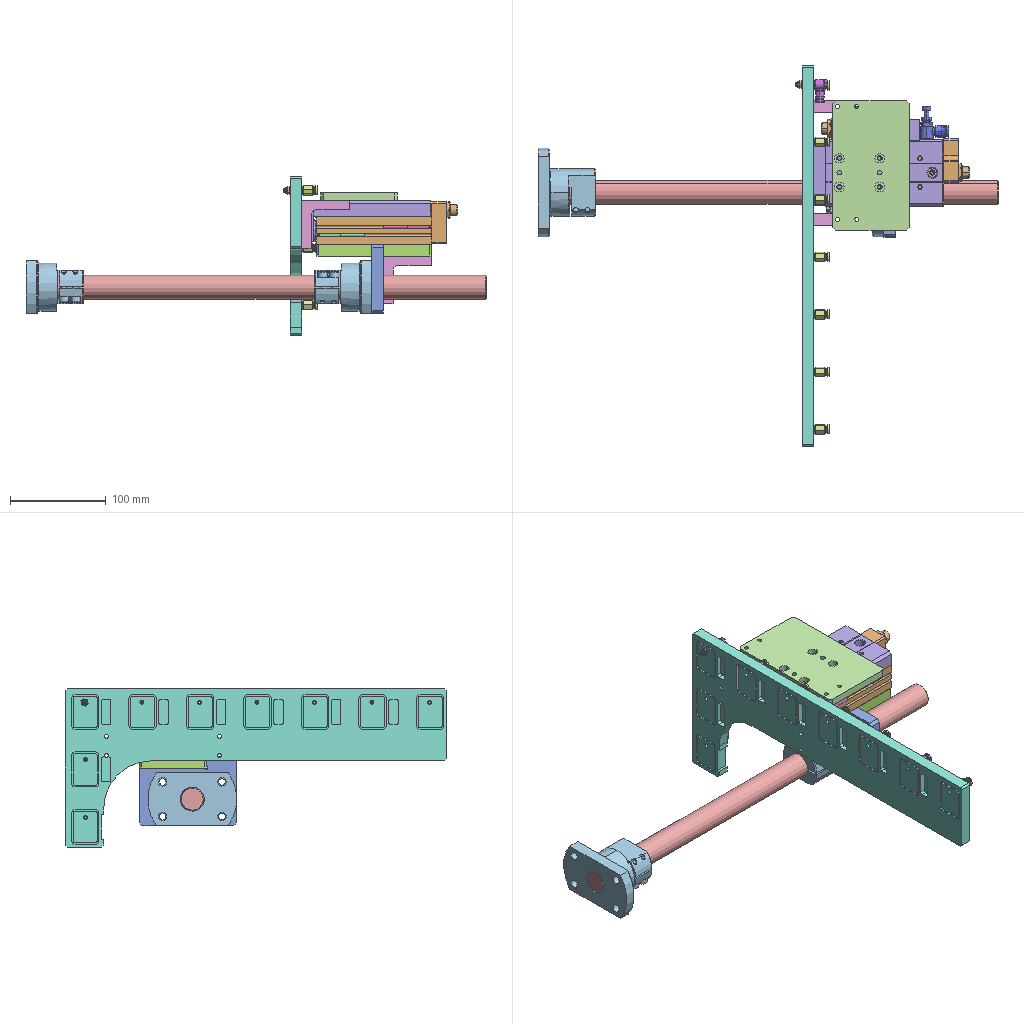Assembly | SolidWorks | 12 different items | 34 placed | box 480 x 398 x 165 mm
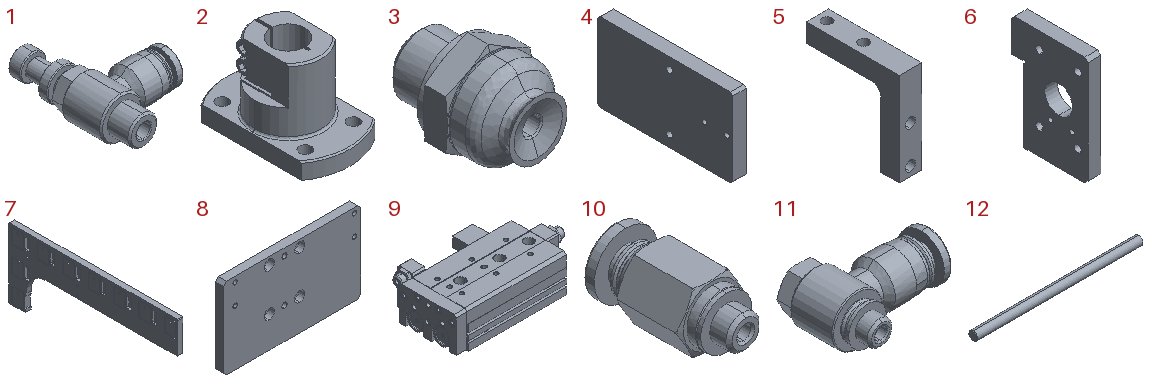Parts list (item | quantity | size | volume | features):
1 | x2 | 30 x 41.5 x 14 mm | 4764 mm3 | features BaseBody 1
2 | x2 | 55 x 93 x 60 mm | 106506 mm3 | features BaseBody 1
3 | x12 | 7 x 10 x 8.083 mm | 260.959 mm3 | features BaseBody 2
4 | x1 | 12 x 120 x 70 mm | 98575 mm3 | features HoleWzd 4, Chamfer 1, Extrusion 1
5 | x3 | 12 x 50 x 50 mm | 9914 mm3 | features HoleWzd 2, Extrusion 1, Fillet 1
6 | x1 | 12 x 72 x 102 mm | 69020 mm3 | features HoleWzd 3, Cut 2, Chamfer 1, Extrusion 1
7 | x1 | 12 x 398 x 165 mm | 392950 mm3 | features ICE 9, LPattern 7, HoleWzd 6, Fillet 4, Cut 3, Chamfer 2, Extrusion 1
8 | x1 | 135 x 8 x 80 mm | 83489 mm3 | features HoleWzd 3, Chamfer 1, Extrusion 1
9 | x1 | 163 x 91 x 46 mm | 387312 mm3 | features BaseBody 4
10 | x8 | 10.392 x 19.5 x 9.5 mm | 848.71 mm3 | features BaseBody 1
11 | x1 | 24.119 x 17 x 10.238 mm | 1557 mm3 | features BaseBody 1
12 | x1 | 480 x 25 x 25 mm | 235543 mm3 | features Chamfer 1, Extrusion 1
Mates (type | each side: item.copy, entity, surface, feature):
Concentric | 12.1 face cylinder Boss-Extrude1 | 2.1 face cylinder Input1
Concentric | 2.2 face cylinder Input1 | 12.1 face cylinder Boss-Extrude1
Coincident | 2.2 face plane Input1 | 12.1 face plane Boss-Extrude1
Concentric | 12.1 face cylinder Boss-Extrude1 | 6.1 face cylinder Cut-Extrude1
Coincident | 2.1 face plane Input1 | 6.1 face plane Boss-Extrude1
DistanceDim | 6.1 face plane Boss-Extrude1 | 2.2 face plane Input1
Coincident | 6.1 face plane Boss-Extrude1 | 4.1 face plane Boss-Extrude1 | 2 times
Coincident | 4.1 face plane Boss-Extrude1 | 5.1 face plane Boss-Extrude1 | 2 times
Width | 4.1 face plane Boss-Extrude1 | 4.1 face plane Boss-Extrude1 | 5.1 face plane Boss-Extrude1 | 5.1 face plane Boss-Extrude1
Coincident | 6.1 face plane Boss-Extrude1 | 5.1 face plane Boss-Extrude1
Parallel | 2.2 face plane Input1 | 6.1 face plane Boss-Extrude1
Coincident | 4.1 face plane Boss-Extrude1 | 9.1 face plane _HLQ20X50-S-A-body-1-solid1 | 2 times
Width | 9.1 face plane _HLQ20X50-S-A-body-1-solid1 | 9.1 face plane _HLQ20X50-S-A-body-1-solid1 | 4.1 face plane Boss-Extrude1 | 4.1 face plane Boss-Extrude1
Coincident | 7.1 face plane Boss-Extrude1 | 9.1 face plane _HLQ20X50-S-A-0-rod-1-solid1
Concentric | 7.1 face cylinder M5 Tapped Hole2 | 10.1 face cylinder Input1
Coincident | 7.1 face plane Boss-Extrude1 | 10.1 face plane Input1
Concentric | 7.1 face cylinder LPattern5 | 10.2 face cylinder Input1
Coincident | 7.1 face plane Boss-Extrude1 | 10.2 face plane Input1
Concentric | 7.1 face cylinder LPattern4 | 11.1 face cylinder Input1
Coincident | 7.1 face plane Boss-Extrude1 | 11.1 face plane Input1
Parallel | 7.1 face plane Boss-Extrude1 | 11.1 face plane Input1
Concentric | 11.1 face cylinder Input1 | 3.1 face cylinder _ZP2-B04EUGS_PAD-1-solid1
Coincident | 7.1 face plane Boss-Extrude1 | 3.1 face plane _ZP2A-Z01P-1-solid1
Concentric | 9.1 face cylinder _HLQ20X50-S-A-body-1-solid1 | 1.1 face cylinder Input1
Coincident | 9.1 face plane _HLQ20X50-S-A-body-1-solid1 | 1.1 face plane Input1
Parallel | 9.1 face plane _HLQ20X50-S-A-body-1-solid1 | 1.1 face plane Input1
Concentric | 9.1 face cylinder _HLQ20X50-S-A-body-1-solid1 | 1.2 face cylinder Input1
Coincident | 9.1 face plane _HLQ20X50-S-A-body-1-solid1 | 1.2 face plane Input1
Parallel | 4.1 face plane Boss-Extrude1 | 1.2 face plane Input1
Parallel | 6.1 face plane Boss-Extrude1 | 2.1 face plane Input1
DistanceDim | 7.1 face plane Boss-Extrude1 | 9.1 face plane _HLQ20X50-S-A-0-rod-1-solid1
Coincident | 9.1 face plane _HLQ20X50-S-A-0-rod-1-solid1 | 8.1 face plane Boss-Extrude1
DistanceDim | 9.1 face plane _HLQ20X50-S-A-0-rod-1-solid1 | 8.1 face plane Boss-Extrude1
DistanceDim | 8.1 face plane Boss-Extrude1 | 9.1 face plane _HLQ20X50-S-A-0-rod-1-solid1
Coincident | 7.1 face plane Boss-Extrude1 | 5.2 face plane Boss-Extrude1
Coincident | 8.1 face plane Boss-Extrude1 | 5.2 face plane Boss-Extrude1 | 2 times
Coincident | 8.1 face plane Boss-Extrude1 | 5.3 face plane Boss-Extrude1
Coincident | 7.1 face plane Boss-Extrude1 | 5.3 face plane Boss-Extrude1
DistanceDim | 5.3 face plane Boss-Extrude1 | 9.1 face plane _HLQ20X50-S-A-0-rod-1-solid1
DistanceDim | 4.1 face plane Boss-Extrude1 | 7.1 face plane Boss-Extrude4